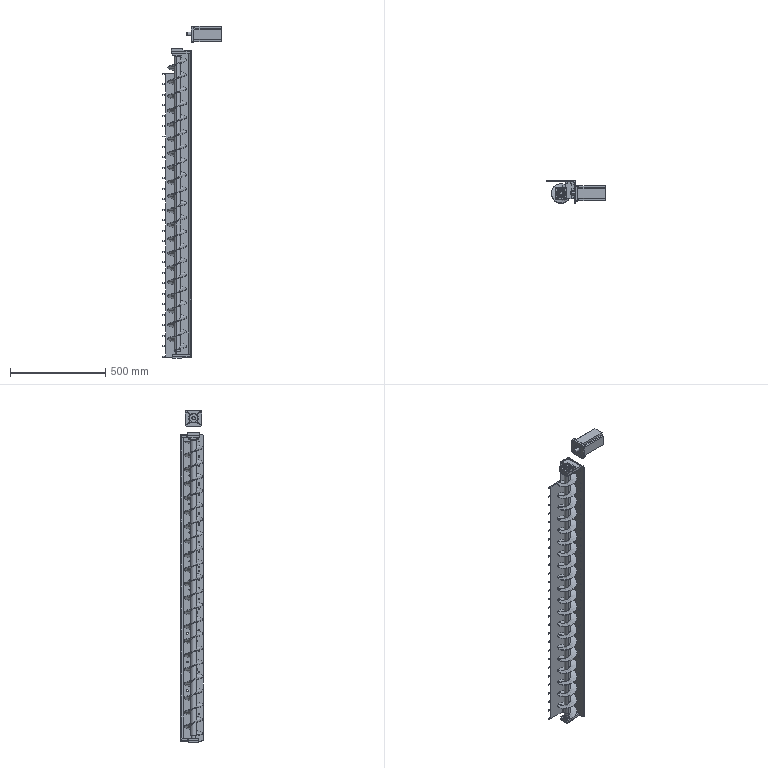Part | SolidWorks | features CompositeCurve 2 | 15 solids | 721 faces | box 307 x 120 x 1742 mm | volume 4354852 mm3 | cylinder 373 | plane 260 | cone 48 | torus 36 | spline 4 | commonest cylinder face diameters 4.2 x86 6.8 x63 5.8 x34 10 x34 5.5 x20 8 x12